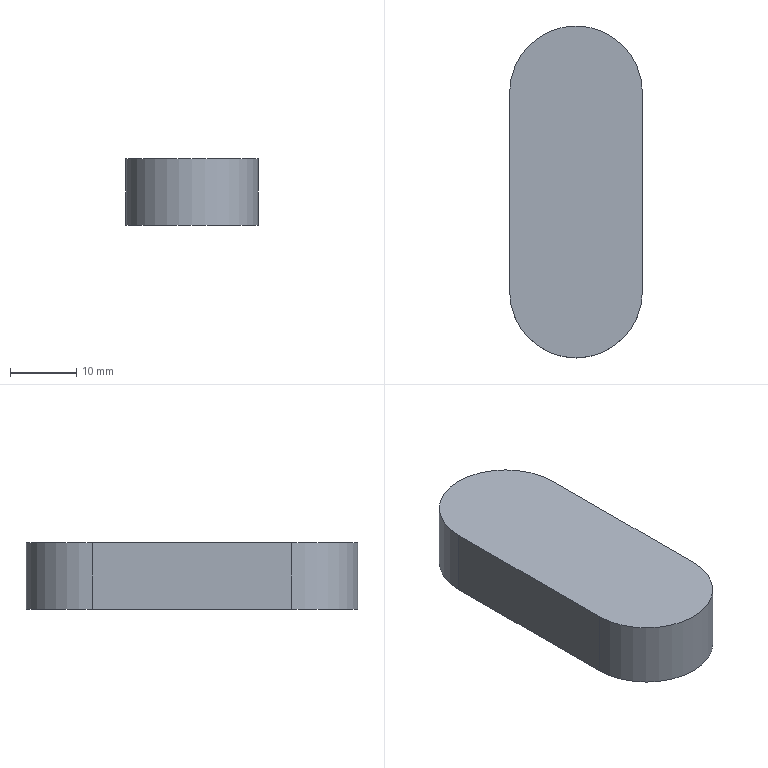Part | NX | features DATUM_CSYS 2, EXTRUDE 1, SKETCH 1 | 1 solid | 6 faces | box 20 x 50 x 10 mm | volume 9142 mm3 | plane 4 | cylinder 2 | commonest cylinder face diameters 20 x2
STEP:
#1=CARTESIAN_POINT('',(-10.,15.,10.));
#2=VERTEX_POINT('',#1);
#3=CARTESIAN_POINT('',(-10.,-15.,10.));
#4=VERTEX_POINT('',#3);
#5=CARTESIAN_POINT('',(-10.,15.,10.));
#6=DIRECTION('',(0.,-1.,0.));
#7=VECTOR('',#6,1000.);
#8=LINE('',#5,#7);
#9=EDGE_CURVE('',#2,#4,#8,.T.);
#10=ORIENTED_EDGE('',*,*,#9,.F.);
#11=CARTESIAN_POINT('',(-10.,15.,0.));
#12=VERTEX_POINT('',#11);
#13=CARTESIAN_POINT('',(-10.,15.,0.));
#14=DIRECTION('',(0.,0.,1.));
#15=VECTOR('',#14,1000.);
#16=LINE('',#13,#15);
#17=EDGE_CURVE('',#12,#2,#16,.T.);
#18=ORIENTED_EDGE('',*,*,#17,.F.);
#19=CARTESIAN_POINT('',(-10.,-15.,0.));
#20=VERTEX_POINT('',#19);
#21=CARTESIAN_POINT('',(-10.,15.,0.));
#22=DIRECTION('',(0.,-1.,0.));
#23=VECTOR('',#22,1000.);
#24=LINE('',#21,#23);
#25=EDGE_CURVE('',#12,#20,#24,.T.);
#26=ORIENTED_EDGE('',*,*,#25,.T.);
#27=CARTESIAN_POINT('',(-10.,-15.,0.));
#28=DIRECTION('',(0.,0.,1.));
#29=VECTOR('',#28,1000.);
#30=LINE('',#27,#29);
#31=EDGE_CURVE('',#20,#4,#30,.T.);
#32=ORIENTED_EDGE('',*,*,#31,.T.);
#33=EDGE_LOOP('',(#10,#18,#26,#32));
#34=FACE_BOUND('',#33,.T.);
#35=CARTESIAN_POINT('',(-10.,15.,0.));
#36=DIRECTION('',(-1.,0.,0.));
#37=DIRECTION('',(0.,0.,1.));
#38=AXIS2_PLACEMENT_3D('',#35,#36,#37);
#39=PLANE('',#38);
#40=ADVANCED_FACE('',(#34),#39,.T.);
#41=CARTESIAN_POINT('',(10.,-15.,10.));
#42=VERTEX_POINT('',#41);
#43=CARTESIAN_POINT('',(0.,-15.,10.));
#44=DIRECTION('',(0.,0.,1.));
#45=DIRECTION('',(1.,0.,0.));
#46=AXIS2_PLACEMENT_3D('',#43,#44,#45);
#47=CIRCLE('',#46,10.);
#48=EDGE_CURVE('',#4,#42,#47,.T.);
#49=ORIENTED_EDGE('',*,*,#48,.F.);
#50=ORIENTED_EDGE('',*,*,#31,.F.);
#51=CARTESIAN_POINT('',(10.,-15.,0.));
#52=VERTEX_POINT('',#51);
#53=CARTESIAN_POINT('',(0.,-15.,0.));
#54=DIRECTION('',(0.,0.,1.));
#55=DIRECTION('',(1.,0.,0.));
#56=AXIS2_PLACEMENT_3D('',#53,#54,#55);
#57=CIRCLE('',#56,10.);
#58=EDGE_CURVE('',#20,#52,#57,.T.);
#59=ORIENTED_EDGE('',*,*,#58,.T.);
#60=CARTESIAN_POINT('',(10.,-15.,0.));
#61=DIRECTION('',(0.,0.,1.));
#62=VECTOR('',#61,1000.);
#63=LINE('',#60,#62);
#64=EDGE_CURVE('',#52,#42,#63,.T.);
#65=ORIENTED_EDGE('',*,*,#64,.T.);
#66=EDGE_LOOP('',(#49,#50,#59,#65));
#67=FACE_BOUND('',#66,.T.);
#68=CARTESIAN_POINT('',(0.,-15.,0.));
#69=DIRECTION('',(0.,0.,1.));
#70=DIRECTION('',(1.,0.,0.));
#71=AXIS2_PLACEMENT_3D('',#68,#69,#70);
#72=CYLINDRICAL_SURFACE('',#71,10.);
#73=ADVANCED_FACE('',(#67),#72,.T.);
#74=CARTESIAN_POINT('',(10.,15.,10.));
#75=VERTEX_POINT('',#74);
#76=CARTESIAN_POINT('',(10.,-15.,10.));
#77=DIRECTION('',(0.,1.,0.));
#78=VECTOR('',#77,1000.);
#79=LINE('',#76,#78);
#80=EDGE_CURVE('',#42,#75,#79,.T.);
#81=ORIENTED_EDGE('',*,*,#80,.F.);
#82=ORIENTED_EDGE('',*,*,#64,.F.);
#83=CARTESIAN_POINT('',(10.,15.,0.));
#84=VERTEX_POINT('',#83);
#85=CARTESIAN_POINT('',(10.,-15.,0.));
#86=DIRECTION('',(0.,1.,0.));
#87=VECTOR('',#86,1000.);
#88=LINE('',#85,#87);
#89=EDGE_CURVE('',#52,#84,#88,.T.);
#90=ORIENTED_EDGE('',*,*,#89,.T.);
#91=CARTESIAN_POINT('',(10.,15.,0.));
#92=DIRECTION('',(0.,0.,1.));
#93=VECTOR('',#92,1000.);
#94=LINE('',#91,#93);
#95=EDGE_CURVE('',#84,#75,#94,.T.);
#96=ORIENTED_EDGE('',*,*,#95,.T.);
#97=EDGE_LOOP('',(#81,#82,#90,#96));
#98=FACE_BOUND('',#97,.T.);
#99=CARTESIAN_POINT('',(10.,-15.,0.));
#100=DIRECTION('',(1.,0.,0.));
#101=DIRECTION('',(0.,0.,-1.));
#102=AXIS2_PLACEMENT_3D('',#99,#100,#101);
#103=PLANE('',#102);
#104=ADVANCED_FACE('',(#98),#103,.T.);
#105=CARTESIAN_POINT('',(0.,15.,10.));
#106=DIRECTION('',(0.,0.,1.));
#107=DIRECTION('',(1.,0.,0.));
#108=AXIS2_PLACEMENT_3D('',#105,#106,#107);
#109=CIRCLE('',#108,10.);
#110=EDGE_CURVE('',#75,#2,#109,.T.);
#111=ORIENTED_EDGE('',*,*,#110,.F.);
#112=ORIENTED_EDGE('',*,*,#95,.F.);
#113=CARTESIAN_POINT('',(0.,15.,0.));
#114=DIRECTION('',(0.,0.,1.));
#115=DIRECTION('',(1.,0.,0.));
#116=AXIS2_PLACEMENT_3D('',#113,#114,#115);
#117=CIRCLE('',#116,10.);
#118=EDGE_CURVE('',#84,#12,#117,.T.);
#119=ORIENTED_EDGE('',*,*,#118,.T.);
#120=ORIENTED_EDGE('',*,*,#17,.T.);
#121=EDGE_LOOP('',(#111,#112,#119,#120));
#122=FACE_BOUND('',#121,.T.);
#123=CARTESIAN_POINT('',(0.,15.,0.));
#124=DIRECTION('',(0.,0.,1.));
#125=DIRECTION('',(1.,0.,0.));
#126=AXIS2_PLACEMENT_3D('',#123,#124,#125);
#127=CYLINDRICAL_SURFACE('',#126,10.);
#128=ADVANCED_FACE('',(#122),#127,.T.);
#129=ORIENTED_EDGE('',*,*,#25,.F.);
#130=ORIENTED_EDGE('',*,*,#118,.F.);
#131=ORIENTED_EDGE('',*,*,#89,.F.);
#132=ORIENTED_EDGE('',*,*,#58,.F.);
#133=EDGE_LOOP('',(#129,#130,#131,#132));
#134=FACE_BOUND('',#133,.T.);
#135=CARTESIAN_POINT('',(0.,-15.,0.));
#136=DIRECTION('',(0.,0.,1.));
#137=DIRECTION('',(1.,0.,0.));
#138=AXIS2_PLACEMENT_3D('',#135,#136,#137);
#139=PLANE('',#138);
#140=ADVANCED_FACE('',(#134),#139,.F.);
#141=ORIENTED_EDGE('',*,*,#9,.T.);
#142=ORIENTED_EDGE('',*,*,#48,.T.);
#143=ORIENTED_EDGE('',*,*,#80,.T.);
#144=ORIENTED_EDGE('',*,*,#110,.T.);
#145=EDGE_LOOP('',(#141,#142,#143,#144));
#146=FACE_BOUND('',#145,.T.);
#147=CARTESIAN_POINT('',(0.,-15.,10.));
#148=DIRECTION('',(0.,0.,1.));
#149=DIRECTION('',(1.,0.,0.));
#150=AXIS2_PLACEMENT_3D('',#147,#148,#149);
#151=PLANE('',#150);
#152=ADVANCED_FACE('',(#146),#151,.T.);
#153=CLOSED_SHELL('',(#40,#73,#104,#128,#140,#152));
#154=MANIFOLD_SOLID_BREP('',#153);
#155=(LENGTH_UNIT()NAMED_UNIT(*)SI_UNIT(.MILLI.,.METRE.));
#156=UNCERTAINTY_MEASURE_WITH_UNIT(LENGTH_MEASURE(0.00001),#155,'','');
#157=(NAMED_UNIT(*)PLANE_ANGLE_UNIT()SI_UNIT($,.RADIAN.));
#158=(NAMED_UNIT(*)SI_UNIT($,.STERADIAN.)SOLID_ANGLE_UNIT());
#159=(GEOMETRIC_REPRESENTATION_CONTEXT(3)GLOBAL_UNCERTAINTY_ASSIGNED_CONTEXT((#156))GLOBAL_UNIT_ASSIGNED_CONTEXT((#155,#157,#158))REPRESENTATION_CONTEXT('',''));
#160=ADVANCED_BREP_SHAPE_REPRESENTATION('',(#154),#159);